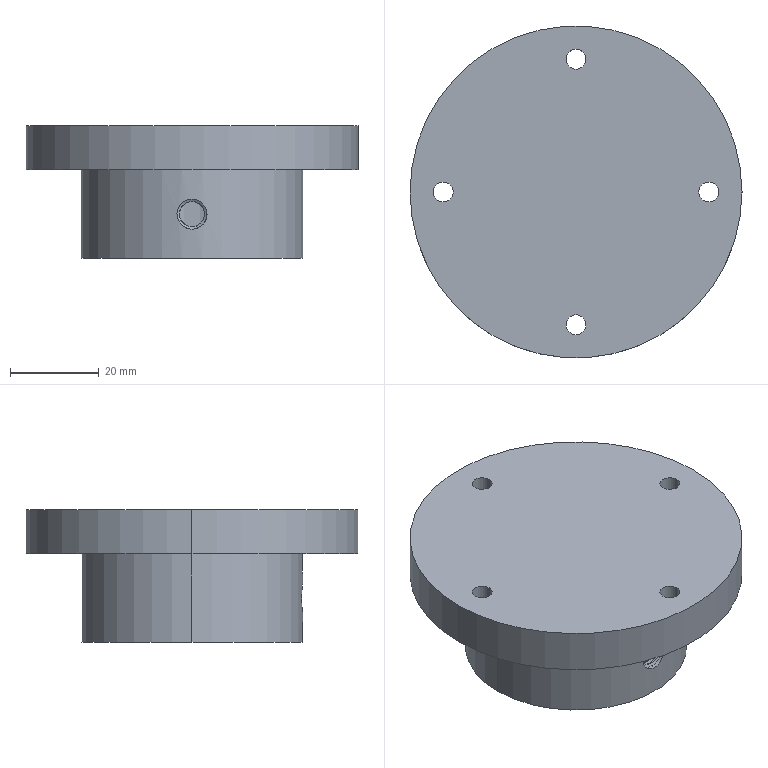Part | SolidWorks | features HoleWzd 2, ICE 2, 3DProfileFeature 1, CirPattern 1, Extrusion 1, SweepThread 1 | 1 solid | 58 faces | box 75 x 75 x 30 mm | volume 67720 mm3 | cylinder 44 | plane 11 | spline 3 | commonest cylinder face diameters 6.8 x20 4.5 x8 8 x8 10 x2 30 x2 50 x2